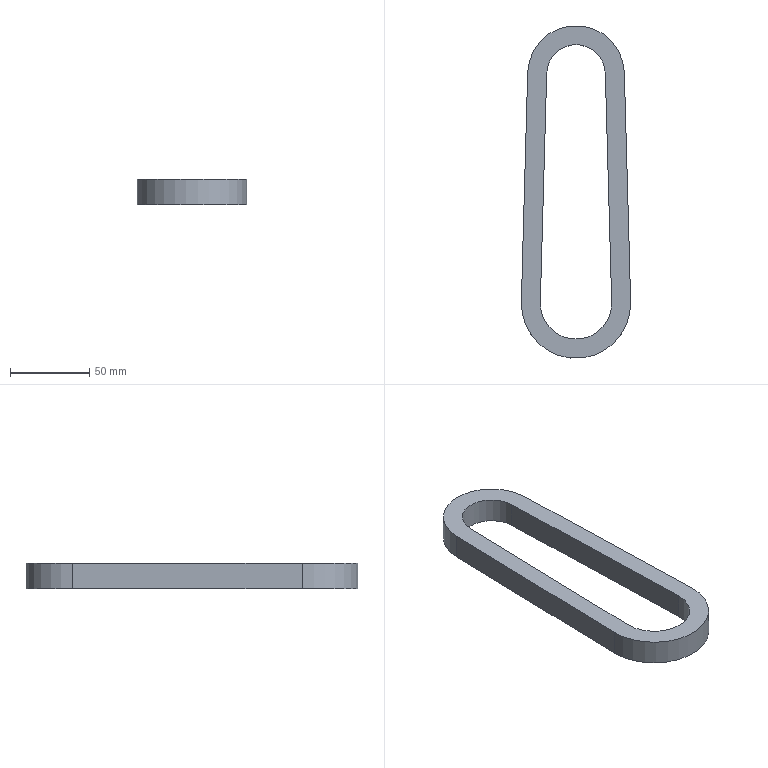Part | NX | features DATUM_CSYS 1, EXTRUDE 1, LINKED_FACE 1, SKETCH 1 | 1 solid | 10 faces | box 69.07 x 210.07 x 16 mm | volume 87712 mm3 | plane 6 | cylinder 4 | commonest cylinder face diameters 37.07 x1 45.07 x1 61.07 x1 69.07 x1
STEP:
#1=CARTESIAN_POINT('',(741.224,-40.171,8.));
#2=VERTEX_POINT('',#1);
#3=CARTESIAN_POINT('',(745.222,104.718,8.));
#4=VERTEX_POINT('',#3);
#5=CARTESIAN_POINT('',(741.224,-40.171,8.));
#6=DIRECTION('',(0.02759,0.9996,0.));
#7=VECTOR('',#6,1000.);
#8=LINE('',#5,#7);
#9=EDGE_CURVE('',#2,#4,#8,.T.);
#10=ORIENTED_EDGE('',*,*,#9,.F.);
#11=CARTESIAN_POINT('',(741.224,-40.171,-8.));
#12=VERTEX_POINT('',#11);
#13=CARTESIAN_POINT('',(741.224,-40.171,-8.));
#14=DIRECTION('',(0.,0.,1.));
#15=VECTOR('',#14,1000.);
#16=LINE('',#13,#15);
#17=EDGE_CURVE('',#12,#2,#16,.T.);
#18=ORIENTED_EDGE('',*,*,#17,.F.);
#19=CARTESIAN_POINT('',(745.222,104.718,-8.));
#20=VERTEX_POINT('',#19);
#21=CARTESIAN_POINT('',(741.224,-40.171,-8.));
#22=DIRECTION('',(0.02759,0.9996,0.));
#23=VECTOR('',#22,1000.);
#24=LINE('',#21,#23);
#25=EDGE_CURVE('',#12,#20,#24,.T.);
#26=ORIENTED_EDGE('',*,*,#25,.T.);
#27=CARTESIAN_POINT('',(745.222,104.718,-8.));
#28=DIRECTION('',(0.,0.,1.));
#29=VECTOR('',#28,1000.);
#30=LINE('',#27,#29);
#31=EDGE_CURVE('',#20,#4,#30,.T.);
#32=ORIENTED_EDGE('',*,*,#31,.T.);
#33=EDGE_LOOP('',(#10,#18,#26,#32));
#34=FACE_BOUND('',#33,.T.);
#35=CARTESIAN_POINT('',(741.224,-40.171,-8.));
#36=DIRECTION('',(0.9996,-0.02759,0.));
#37=DIRECTION('',(0.02759,0.9996,0.));
#38=AXIS2_PLACEMENT_3D('',#35,#36,#37);
#39=PLANE('',#38);
#40=ADVANCED_FACE('',(#34),#39,.T.);
#41=CARTESIAN_POINT('',(782.278,104.718,8.));
#42=VERTEX_POINT('',#41);
#43=CARTESIAN_POINT('',(763.75,104.207,8.));
#44=DIRECTION('',(0.,0.,-1.));
#45=DIRECTION('',(-0.9996,0.02759,0.));
#46=AXIS2_PLACEMENT_3D('',#43,#44,#45);
#47=CIRCLE('',#46,18.535);
#48=EDGE_CURVE('',#4,#42,#47,.T.);
#49=ORIENTED_EDGE('',*,*,#48,.F.);
#50=ORIENTED_EDGE('',*,*,#31,.F.);
#51=CARTESIAN_POINT('',(782.278,104.718,-8.));
#52=VERTEX_POINT('',#51);
#53=CARTESIAN_POINT('',(763.75,104.207,-8.));
#54=DIRECTION('',(0.,0.,-1.));
#55=DIRECTION('',(-0.9996,0.02759,0.));
#56=AXIS2_PLACEMENT_3D('',#53,#54,#55);
#57=CIRCLE('',#56,18.535);
#58=EDGE_CURVE('',#20,#52,#57,.T.);
#59=ORIENTED_EDGE('',*,*,#58,.T.);
#60=CARTESIAN_POINT('',(782.278,104.718,-8.));
#61=DIRECTION('',(0.,0.,1.));
#62=VECTOR('',#61,1000.);
#63=LINE('',#60,#62);
#64=EDGE_CURVE('',#52,#42,#63,.T.);
#65=ORIENTED_EDGE('',*,*,#64,.T.);
#66=EDGE_LOOP('',(#49,#50,#59,#65));
#67=FACE_BOUND('',#66,.T.);
#68=CARTESIAN_POINT('',(763.75,104.207,-8.));
#69=DIRECTION('',(0.,0.,1.));
#70=DIRECTION('',(1.,0.,0.));
#71=AXIS2_PLACEMENT_3D('',#68,#69,#70);
#72=CYLINDRICAL_SURFACE('',#71,18.535);
#73=ADVANCED_FACE('',(#67),#72,.F.);
#74=CARTESIAN_POINT('',(786.276,-40.171,8.));
#75=VERTEX_POINT('',#74);
#76=CARTESIAN_POINT('',(782.278,104.718,8.));
#77=DIRECTION('',(0.02759,-0.9996,0.));
#78=VECTOR('',#77,1000.);
#79=LINE('',#76,#78);
#80=EDGE_CURVE('',#42,#75,#79,.T.);
#81=ORIENTED_EDGE('',*,*,#80,.F.);
#82=ORIENTED_EDGE('',*,*,#64,.F.);
#83=CARTESIAN_POINT('',(786.276,-40.171,-8.));
#84=VERTEX_POINT('',#83);
#85=CARTESIAN_POINT('',(782.278,104.718,-8.));
#86=DIRECTION('',(0.02759,-0.9996,0.));
#87=VECTOR('',#86,1000.);
#88=LINE('',#85,#87);
#89=EDGE_CURVE('',#52,#84,#88,.T.);
#90=ORIENTED_EDGE('',*,*,#89,.T.);
#91=CARTESIAN_POINT('',(786.276,-40.171,-8.));
#92=DIRECTION('',(0.,0.,1.));
#93=VECTOR('',#92,1000.);
#94=LINE('',#91,#93);
#95=EDGE_CURVE('',#84,#75,#94,.T.);
#96=ORIENTED_EDGE('',*,*,#95,.T.);
#97=EDGE_LOOP('',(#81,#82,#90,#96));
#98=FACE_BOUND('',#97,.T.);
#99=CARTESIAN_POINT('',(782.278,104.718,-8.));
#100=DIRECTION('',(-0.9996,-0.02759,0.));
#101=DIRECTION('',(0.02759,-0.9996,0.));
#102=AXIS2_PLACEMENT_3D('',#99,#100,#101);
#103=PLANE('',#102);
#104=ADVANCED_FACE('',(#98),#103,.T.);
#105=CARTESIAN_POINT('',(729.228,-39.84,8.));
#106=VERTEX_POINT('',#105);
#107=CARTESIAN_POINT('',(798.272,-39.84,8.));
#108=VERTEX_POINT('',#107);
#109=CARTESIAN_POINT('',(763.75,-40.793,8.));
#110=DIRECTION('',(0.,0.,1.));
#111=DIRECTION('',(1.,0.,0.));
#112=AXIS2_PLACEMENT_3D('',#109,#110,#111);
#113=CIRCLE('',#112,34.535);
#114=EDGE_CURVE('',#106,#108,#113,.T.);
#115=ORIENTED_EDGE('',*,*,#114,.F.);
#116=CARTESIAN_POINT('',(729.228,-39.84,-8.));
#117=VERTEX_POINT('',#116);
#118=CARTESIAN_POINT('',(729.228,-39.84,-8.));
#119=DIRECTION('',(0.,0.,1.));
#120=VECTOR('',#119,1000.);
#121=LINE('',#118,#120);
#122=EDGE_CURVE('',#117,#106,#121,.T.);
#123=ORIENTED_EDGE('',*,*,#122,.F.);
#124=CARTESIAN_POINT('',(798.272,-39.84,-8.));
#125=VERTEX_POINT('',#124);
#126=CARTESIAN_POINT('',(763.75,-40.793,-8.));
#127=DIRECTION('',(0.,0.,1.));
#128=DIRECTION('',(-0.9996,0.02759,0.));
#129=AXIS2_PLACEMENT_3D('',#126,#127,#128);
#130=CIRCLE('',#129,34.535);
#131=EDGE_CURVE('',#117,#125,#130,.T.);
#132=ORIENTED_EDGE('',*,*,#131,.T.);
#133=CARTESIAN_POINT('',(798.272,-39.84,-8.));
#134=DIRECTION('',(0.,0.,1.));
#135=VECTOR('',#134,1000.);
#136=LINE('',#133,#135);
#137=EDGE_CURVE('',#125,#108,#136,.T.);
#138=ORIENTED_EDGE('',*,*,#137,.T.);
#139=EDGE_LOOP('',(#115,#123,#132,#138));
#140=FACE_BOUND('',#139,.T.);
#141=CARTESIAN_POINT('',(763.75,-40.793,-8.));
#142=DIRECTION('',(0.,0.,1.));
#143=DIRECTION('',(1.,0.,0.));
#144=AXIS2_PLACEMENT_3D('',#141,#142,#143);
#145=CYLINDRICAL_SURFACE('',#144,34.535);
#146=ADVANCED_FACE('',(#140),#145,.T.);
#147=CARTESIAN_POINT('',(794.273,105.049,8.));
#148=VERTEX_POINT('',#147);
#149=CARTESIAN_POINT('',(798.272,-39.84,8.));
#150=DIRECTION('',(-0.02759,0.9996,0.));
#151=VECTOR('',#150,1000.);
#152=LINE('',#149,#151);
#153=EDGE_CURVE('',#108,#148,#152,.T.);
#154=ORIENTED_EDGE('',*,*,#153,.F.);
#155=ORIENTED_EDGE('',*,*,#137,.F.);
#156=CARTESIAN_POINT('',(794.273,105.049,-8.));
#157=VERTEX_POINT('',#156);
#158=CARTESIAN_POINT('',(798.272,-39.84,-8.));
#159=DIRECTION('',(-0.02759,0.9996,0.));
#160=VECTOR('',#159,1000.);
#161=LINE('',#158,#160);
#162=EDGE_CURVE('',#125,#157,#161,.T.);
#163=ORIENTED_EDGE('',*,*,#162,.T.);
#164=CARTESIAN_POINT('',(794.273,105.049,-8.));
#165=DIRECTION('',(0.,0.,1.));
#166=VECTOR('',#165,1000.);
#167=LINE('',#164,#166);
#168=EDGE_CURVE('',#157,#148,#167,.T.);
#169=ORIENTED_EDGE('',*,*,#168,.T.);
#170=EDGE_LOOP('',(#154,#155,#163,#169));
#171=FACE_BOUND('',#170,.T.);
#172=CARTESIAN_POINT('',(798.272,-39.84,-8.));
#173=DIRECTION('',(0.9996,0.02759,0.));
#174=DIRECTION('',(-0.02759,0.9996,0.));
#175=AXIS2_PLACEMENT_3D('',#172,#173,#174);
#176=PLANE('',#175);
#177=ADVANCED_FACE('',(#171),#176,.T.);
#178=CARTESIAN_POINT('',(733.227,105.049,8.));
#179=VERTEX_POINT('',#178);
#180=CARTESIAN_POINT('',(763.75,104.207,8.));
#181=DIRECTION('',(0.,0.,1.));
#182=DIRECTION('',(0.9996,0.02759,0.));
#183=AXIS2_PLACEMENT_3D('',#180,#181,#182);
#184=CIRCLE('',#183,30.535);
#185=EDGE_CURVE('',#148,#179,#184,.T.);
#186=ORIENTED_EDGE('',*,*,#185,.F.);
#187=ORIENTED_EDGE('',*,*,#168,.F.);
#188=CARTESIAN_POINT('',(733.227,105.049,-8.));
#189=VERTEX_POINT('',#188);
#190=CARTESIAN_POINT('',(763.75,104.207,-8.));
#191=DIRECTION('',(0.,0.,1.));
#192=DIRECTION('',(0.9996,0.02759,0.));
#193=AXIS2_PLACEMENT_3D('',#190,#191,#192);
#194=CIRCLE('',#193,30.535);
#195=EDGE_CURVE('',#157,#189,#194,.T.);
#196=ORIENTED_EDGE('',*,*,#195,.T.);
#197=CARTESIAN_POINT('',(733.227,105.049,-8.));
#198=DIRECTION('',(0.,0.,1.));
#199=VECTOR('',#198,1000.);
#200=LINE('',#197,#199);
#201=EDGE_CURVE('',#189,#179,#200,.T.);
#202=ORIENTED_EDGE('',*,*,#201,.T.);
#203=EDGE_LOOP('',(#186,#187,#196,#202));
#204=FACE_BOUND('',#203,.T.);
#205=CARTESIAN_POINT('',(763.75,104.207,-8.));
#206=DIRECTION('',(0.,0.,1.));
#207=DIRECTION('',(1.,0.,0.));
#208=AXIS2_PLACEMENT_3D('',#205,#206,#207);
#209=CYLINDRICAL_SURFACE('',#208,30.535);
#210=ADVANCED_FACE('',(#204),#209,.T.);
#211=CARTESIAN_POINT('',(733.227,105.049,8.));
#212=DIRECTION('',(-0.02759,-0.9996,0.));
#213=VECTOR('',#212,1000.);
#214=LINE('',#211,#213);
#215=EDGE_CURVE('',#179,#106,#214,.T.);
#216=ORIENTED_EDGE('',*,*,#215,.F.);
#217=ORIENTED_EDGE('',*,*,#201,.F.);
#218=CARTESIAN_POINT('',(733.227,105.049,-8.));
#219=DIRECTION('',(-0.02759,-0.9996,0.));
#220=VECTOR('',#219,1000.);
#221=LINE('',#218,#220);
#222=EDGE_CURVE('',#189,#117,#221,.T.);
#223=ORIENTED_EDGE('',*,*,#222,.T.);
#224=ORIENTED_EDGE('',*,*,#122,.T.);
#225=EDGE_LOOP('',(#216,#217,#223,#224));
#226=FACE_BOUND('',#225,.T.);
#227=CARTESIAN_POINT('',(733.227,105.049,-8.));
#228=DIRECTION('',(-0.9996,0.02759,0.));
#229=DIRECTION('',(-0.02759,-0.9996,0.));
#230=AXIS2_PLACEMENT_3D('',#227,#228,#229);
#231=PLANE('',#230);
#232=ADVANCED_FACE('',(#226),#231,.T.);
#233=CARTESIAN_POINT('',(763.75,-40.793,8.));
#234=DIRECTION('',(0.,0.,-1.));
#235=DIRECTION('',(1.,0.,0.));
#236=AXIS2_PLACEMENT_3D('',#233,#234,#235);
#237=CIRCLE('',#236,22.535);
#238=EDGE_CURVE('',#75,#2,#237,.T.);
#239=ORIENTED_EDGE('',*,*,#238,.F.);
#240=ORIENTED_EDGE('',*,*,#95,.F.);
#241=CARTESIAN_POINT('',(763.75,-40.793,-8.));
#242=DIRECTION('',(0.,0.,-1.));
#243=DIRECTION('',(-1.,0.,0.));
#244=AXIS2_PLACEMENT_3D('',#241,#242,#243);
#245=CIRCLE('',#244,22.535);
#246=EDGE_CURVE('',#84,#12,#245,.T.);
#247=ORIENTED_EDGE('',*,*,#246,.T.);
#248=ORIENTED_EDGE('',*,*,#17,.T.);
#249=EDGE_LOOP('',(#239,#240,#247,#248));
#250=FACE_BOUND('',#249,.T.);
#251=CARTESIAN_POINT('',(763.75,-40.793,-8.));
#252=DIRECTION('',(0.,0.,1.));
#253=DIRECTION('',(1.,0.,0.));
#254=AXIS2_PLACEMENT_3D('',#251,#252,#253);
#255=CYLINDRICAL_SURFACE('',#254,22.535);
#256=ADVANCED_FACE('',(#250),#255,.F.);
#257=ORIENTED_EDGE('',*,*,#131,.F.);
#258=ORIENTED_EDGE('',*,*,#222,.F.);
#259=ORIENTED_EDGE('',*,*,#195,.F.);
#260=ORIENTED_EDGE('',*,*,#162,.F.);
#261=EDGE_LOOP('',(#257,#258,#259,#260));
#262=FACE_BOUND('',#261,.T.);
#263=ORIENTED_EDGE('',*,*,#246,.F.);
#264=ORIENTED_EDGE('',*,*,#89,.F.);
#265=ORIENTED_EDGE('',*,*,#58,.F.);
#266=ORIENTED_EDGE('',*,*,#25,.F.);
#267=EDGE_LOOP('',(#263,#264,#265,#266));
#268=FACE_BOUND('',#267,.T.);
#269=CARTESIAN_POINT('',(763.75,-40.793,-8.));
#270=DIRECTION('',(0.,0.,1.));
#271=DIRECTION('',(1.,0.,0.));
#272=AXIS2_PLACEMENT_3D('',#269,#270,#271);
#273=PLANE('',#272);
#274=ADVANCED_FACE('',(#262,#268),#273,.F.);
#275=ORIENTED_EDGE('',*,*,#215,.T.);
#276=ORIENTED_EDGE('',*,*,#114,.T.);
#277=ORIENTED_EDGE('',*,*,#153,.T.);
#278=ORIENTED_EDGE('',*,*,#185,.T.);
#279=EDGE_LOOP('',(#275,#276,#277,#278));
#280=FACE_BOUND('',#279,.T.);
#281=ORIENTED_EDGE('',*,*,#238,.T.);
#282=ORIENTED_EDGE('',*,*,#9,.T.);
#283=ORIENTED_EDGE('',*,*,#48,.T.);
#284=ORIENTED_EDGE('',*,*,#80,.T.);
#285=EDGE_LOOP('',(#281,#282,#283,#284));
#286=FACE_BOUND('',#285,.T.);
#287=CARTESIAN_POINT('',(763.75,-40.793,8.));
#288=DIRECTION('',(0.,0.,1.));
#289=DIRECTION('',(1.,0.,0.));
#290=AXIS2_PLACEMENT_3D('',#287,#288,#289);
#291=PLANE('',#290);
#292=ADVANCED_FACE('',(#280,#286),#291,.T.);
#293=CLOSED_SHELL('',(#40,#73,#104,#146,#177,#210,#232,#256,#274,#292));
#294=MANIFOLD_SOLID_BREP('',#293);
#295=(LENGTH_UNIT()NAMED_UNIT(*)SI_UNIT(.MILLI.,.METRE.));
#296=UNCERTAINTY_MEASURE_WITH_UNIT(LENGTH_MEASURE(0.00001),#295,'','');
#297=(NAMED_UNIT(*)PLANE_ANGLE_UNIT()SI_UNIT($,.RADIAN.));
#298=(NAMED_UNIT(*)SI_UNIT($,.STERADIAN.)SOLID_ANGLE_UNIT());
#299=(GEOMETRIC_REPRESENTATION_CONTEXT(3)GLOBAL_UNCERTAINTY_ASSIGNED_CONTEXT((#296))GLOBAL_UNIT_ASSIGNED_CONTEXT((#295,#297,#298))REPRESENTATION_CONTEXT('',''));
#300=ADVANCED_BREP_SHAPE_REPRESENTATION('',(#294),#299);